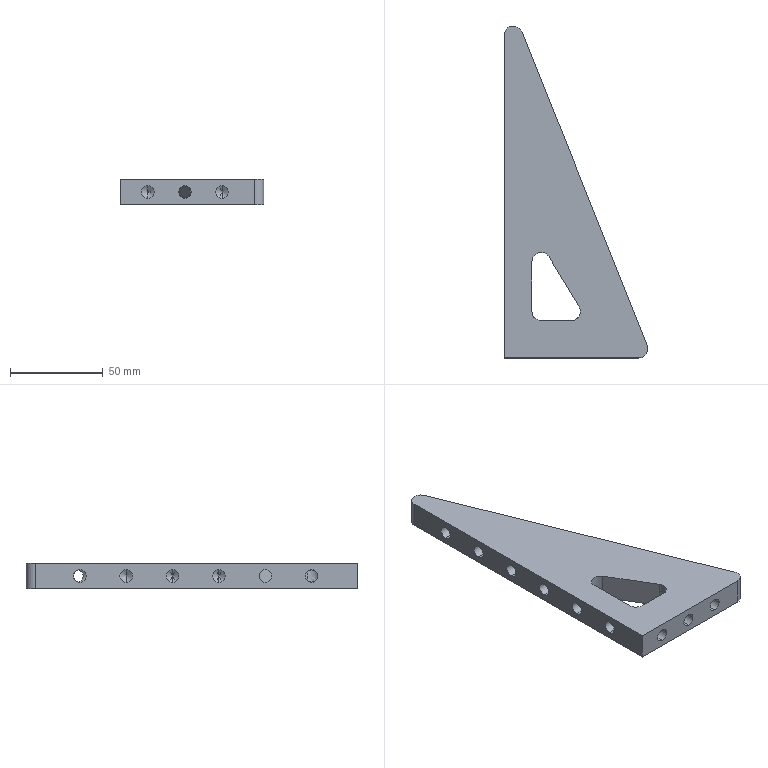Part | STEP file | MT-COMBO-119-S028 | 1 solid | 48 faces | box 77.615 x 179.037 x 14 mm | volume 94866 mm3 | cylinder 24 | cone 15 | plane 8 | spline 1 | commonest cylinder face diameters 6.8 x18 10 x6